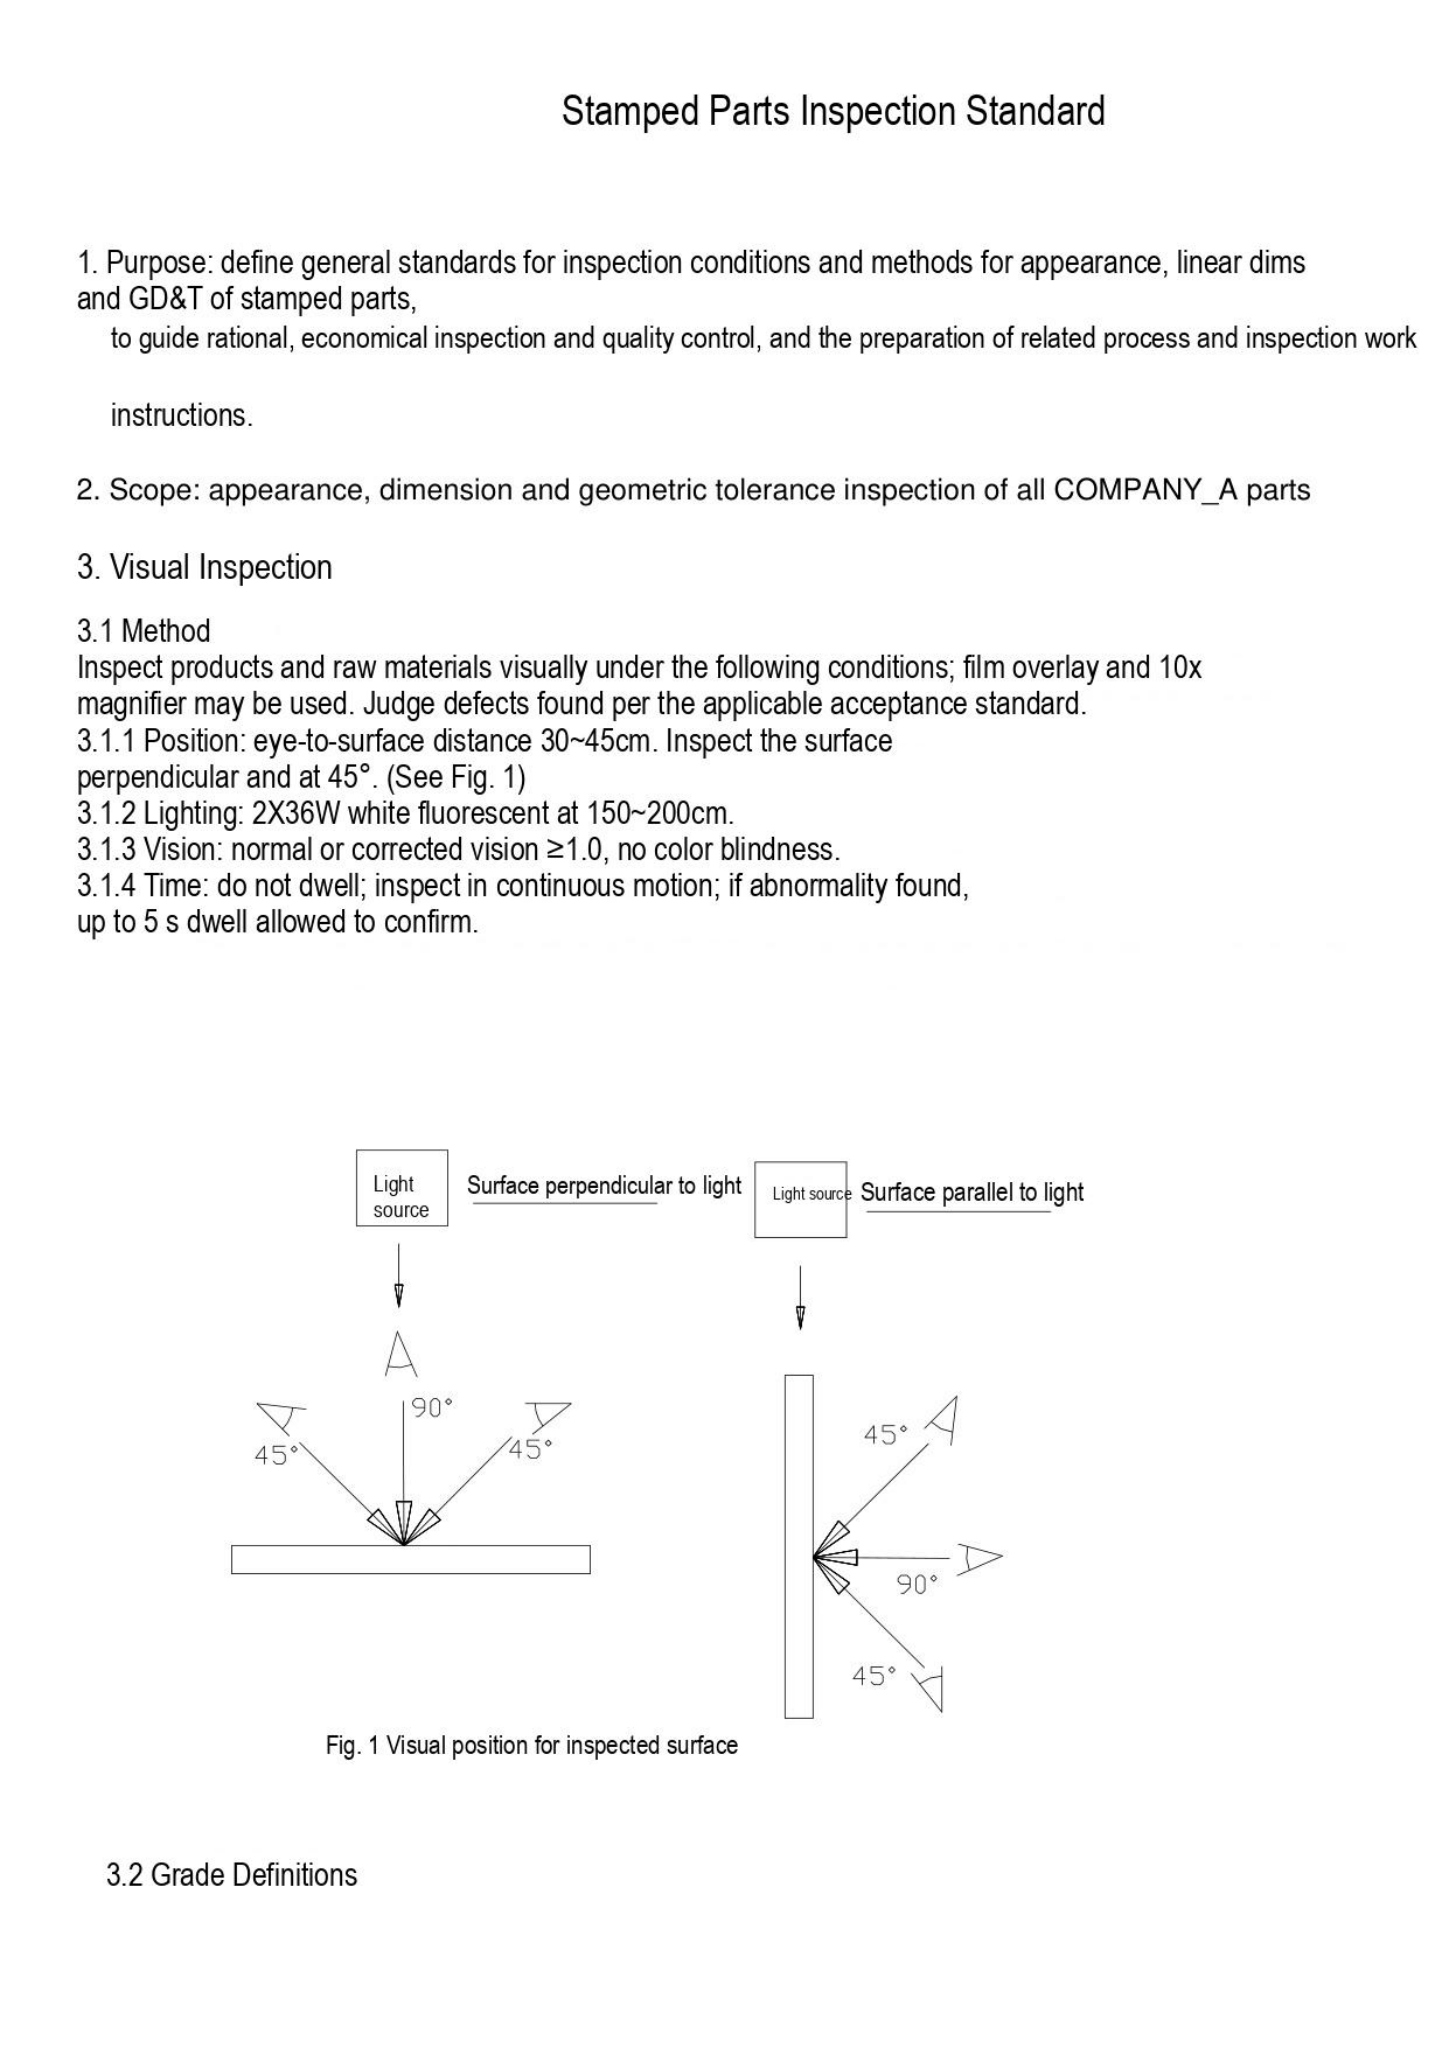Stamped Parts Inspection Standard

1. Purpose: define general standards for inspection conditions and methods for appearance, linear dims and GD&T of stamped parts,
to guide rational, economical inspection and quality control, and the preparation of related process and inspection work instructions.

2. Scope: appearance, dimension and geometric tolerance inspection of all COMPANY_A parts

3. Visual Inspection

3.1 Method
Inspect products and raw materials visually under the following conditions; film overlay and 10x magnifier may be used. Judge defects found per the applicable acceptance standard.
3.1.1 Position: eye-to-surface distance 30~45cm. Inspect the surface perpendicular and at 45°. (See Fig. 1)
3.1.2 Lighting: 2X36W white fluorescent at 150~200cm.
3.1.3 Vision: normal or corrected vision ≥1.0, no color blindness.
3.1.4 Time: do not dwell; inspect in continuous motion; if abnormality found, up to 5 s dwell allowed to confirm.

Light source
Surface perpendicular to light
90°
45°
45°

Light source
Surface parallel to light
45°
90°
45°

Fig. 1 Visual position for inspected surface

3.2 Grade Definitions
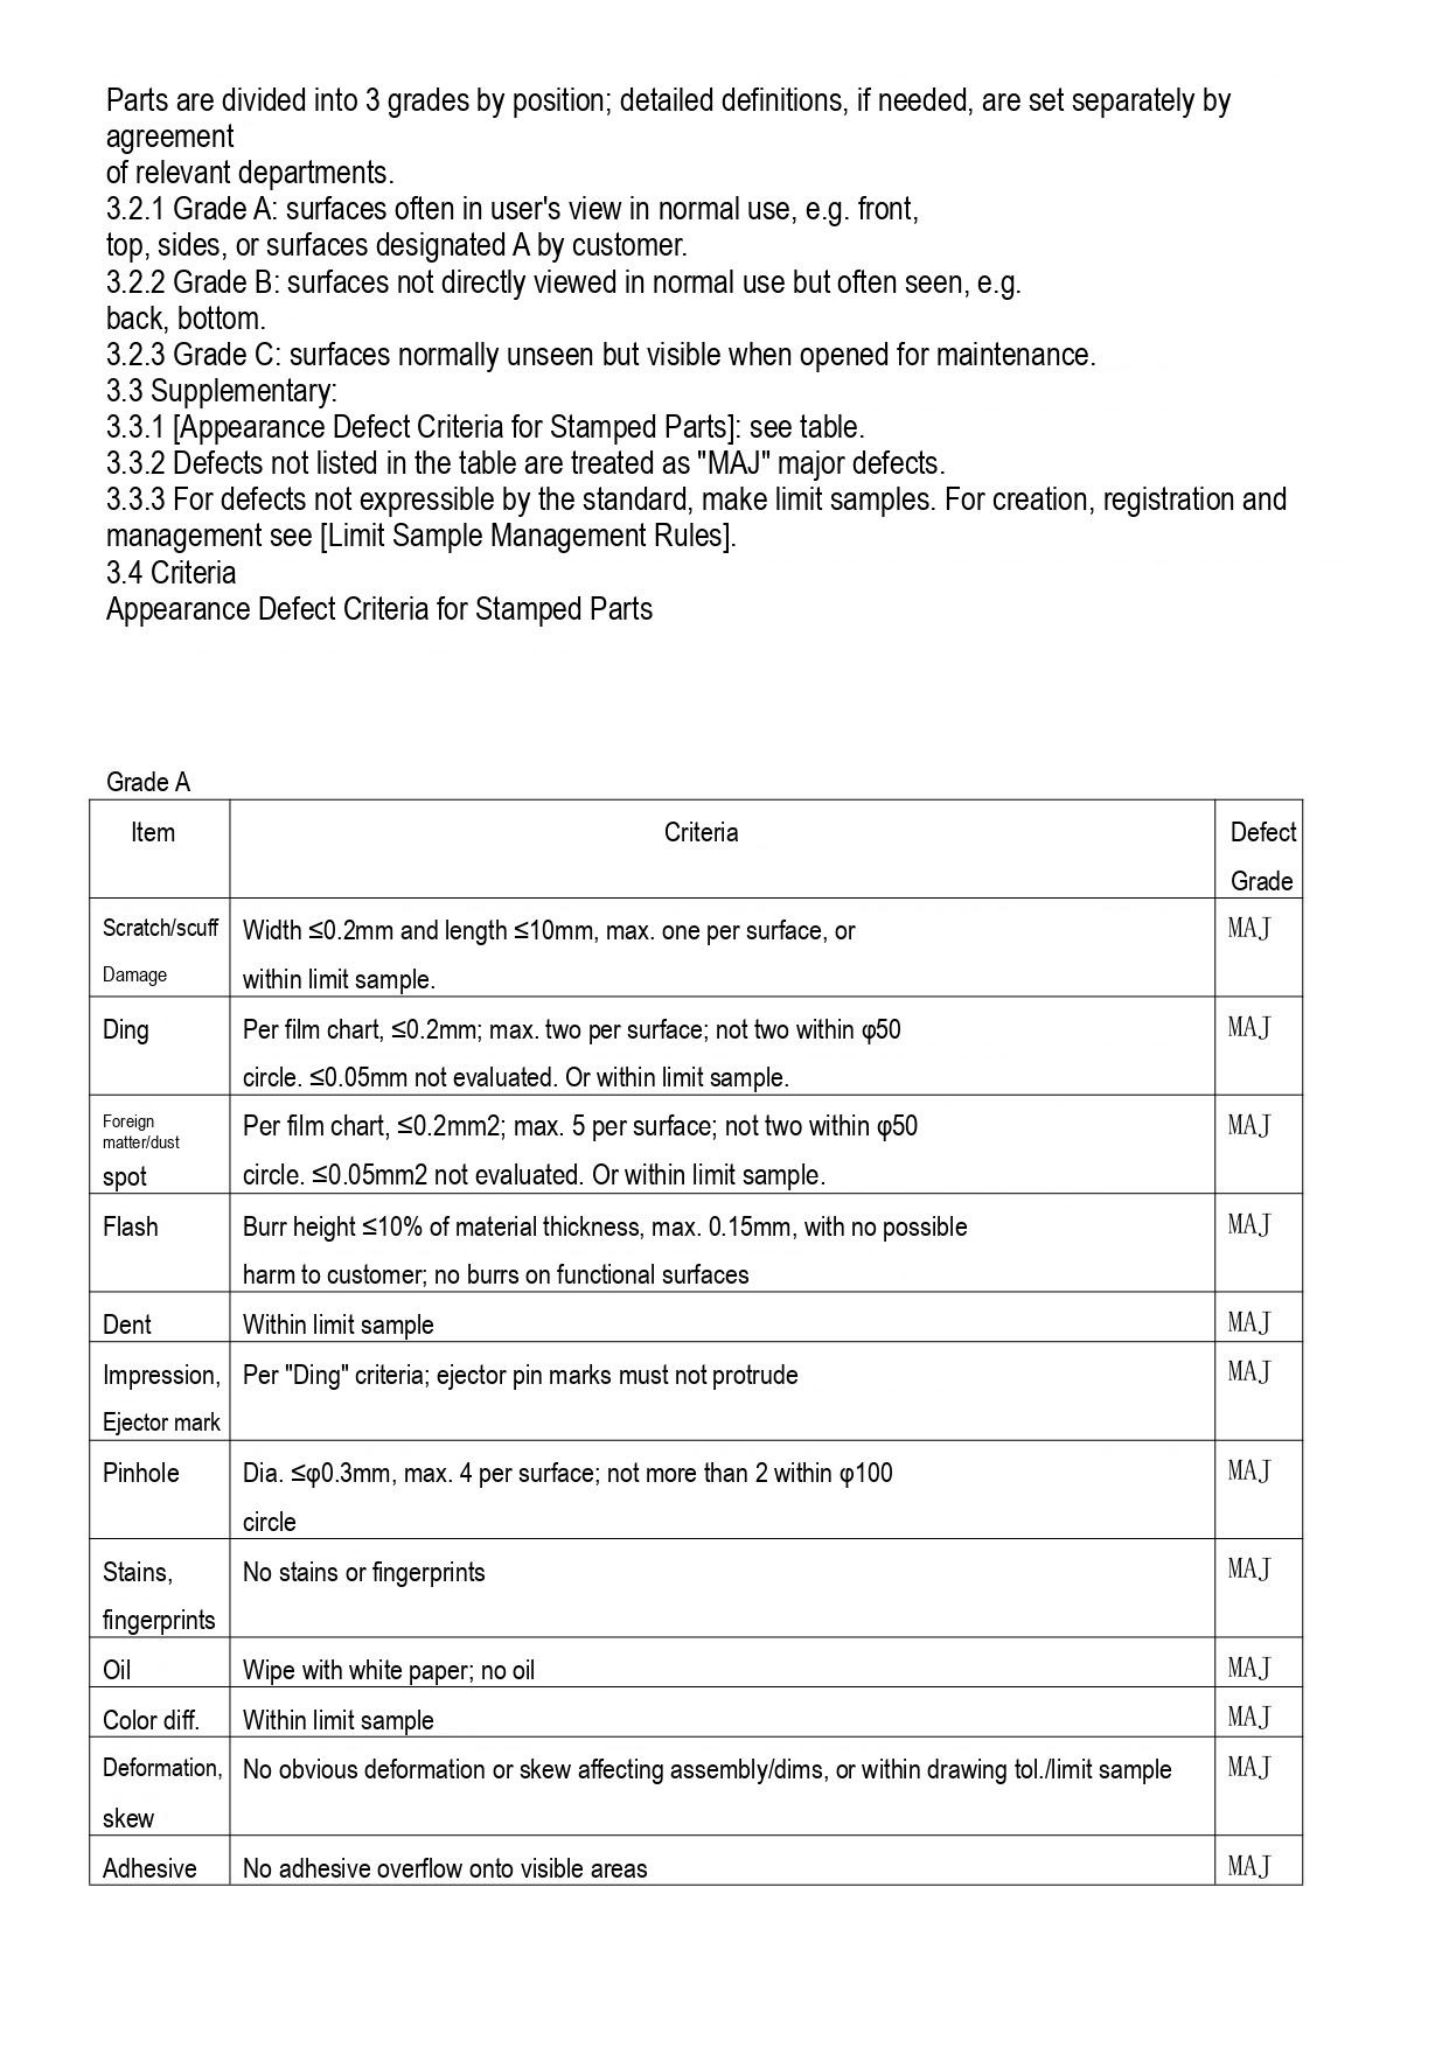Parts are divided into 3 grades by position; detailed definitions, if needed, are set separately by agreement
of relevant departments.
3.2.1 Grade A: surfaces often in user's view in normal use, e.g. front,
top, sides, or surfaces designated A by customer.
3.2.2 Grade B: surfaces not directly viewed in normal use but often seen, e.g.
back, bottom.
3.2.3 Grade C: surfaces normally unseen but visible when opened for maintenance.
3.3 Supplementary:
3.3.1 [Appearance Defect Criteria for Stamped Parts]: see table.
3.3.2 Defects not listed in the table are treated as "MAJ" major defects.
3.3.3 For defects not expressible by the standard, make limit samples. For creation, registration and management see [Limit Sample Management Rules].
3.4 Criteria
Appearance Defect Criteria for Stamped Parts

Grade A

| Item | Criteria | Defect Grade |
|---|---|---|
| Scratch/scuff Damage | Width ≤0.2mm and length ≤10mm, max. one per surface, or within limit sample. | MAJ |
| Ding | Per film chart, ≤0.2mm; max. two per surface; not two within φ50 circle. ≤0.05mm not evaluated. Or within limit sample. | MAJ |
| Foreign matter/dust spot | Per film chart, ≤0.2mm2; max. 5 per surface; not two within φ50 circle. ≤0.05mm2 not evaluated. Or within limit sample. | MAJ |
| Flash | Burr height ≤10% of material thickness, max. 0.15mm, with no possible harm to customer; no burrs on functional surfaces | MAJ |
| Dent | Within limit sample | MAJ |
| Impression, Ejector mark | Per "Ding" criteria; ejector pin marks must not protrude | MAJ |
| Pinhole | Dia. ≤φ0.3mm, max. 4 per surface; not more than 2 within φ100 circle | MAJ |
| Stains, fingerprints | No stains or fingerprints | MAJ |
| Oil | Wipe with white paper; no oil | MAJ |
| Color diff. | Within limit sample | MAJ |
| Deformation, skew | No obvious deformation or skew affecting assembly/dims, or within drawing tol./limit sample | MAJ |
| Adhesive | No adhesive overflow onto visible areas | MAJ |
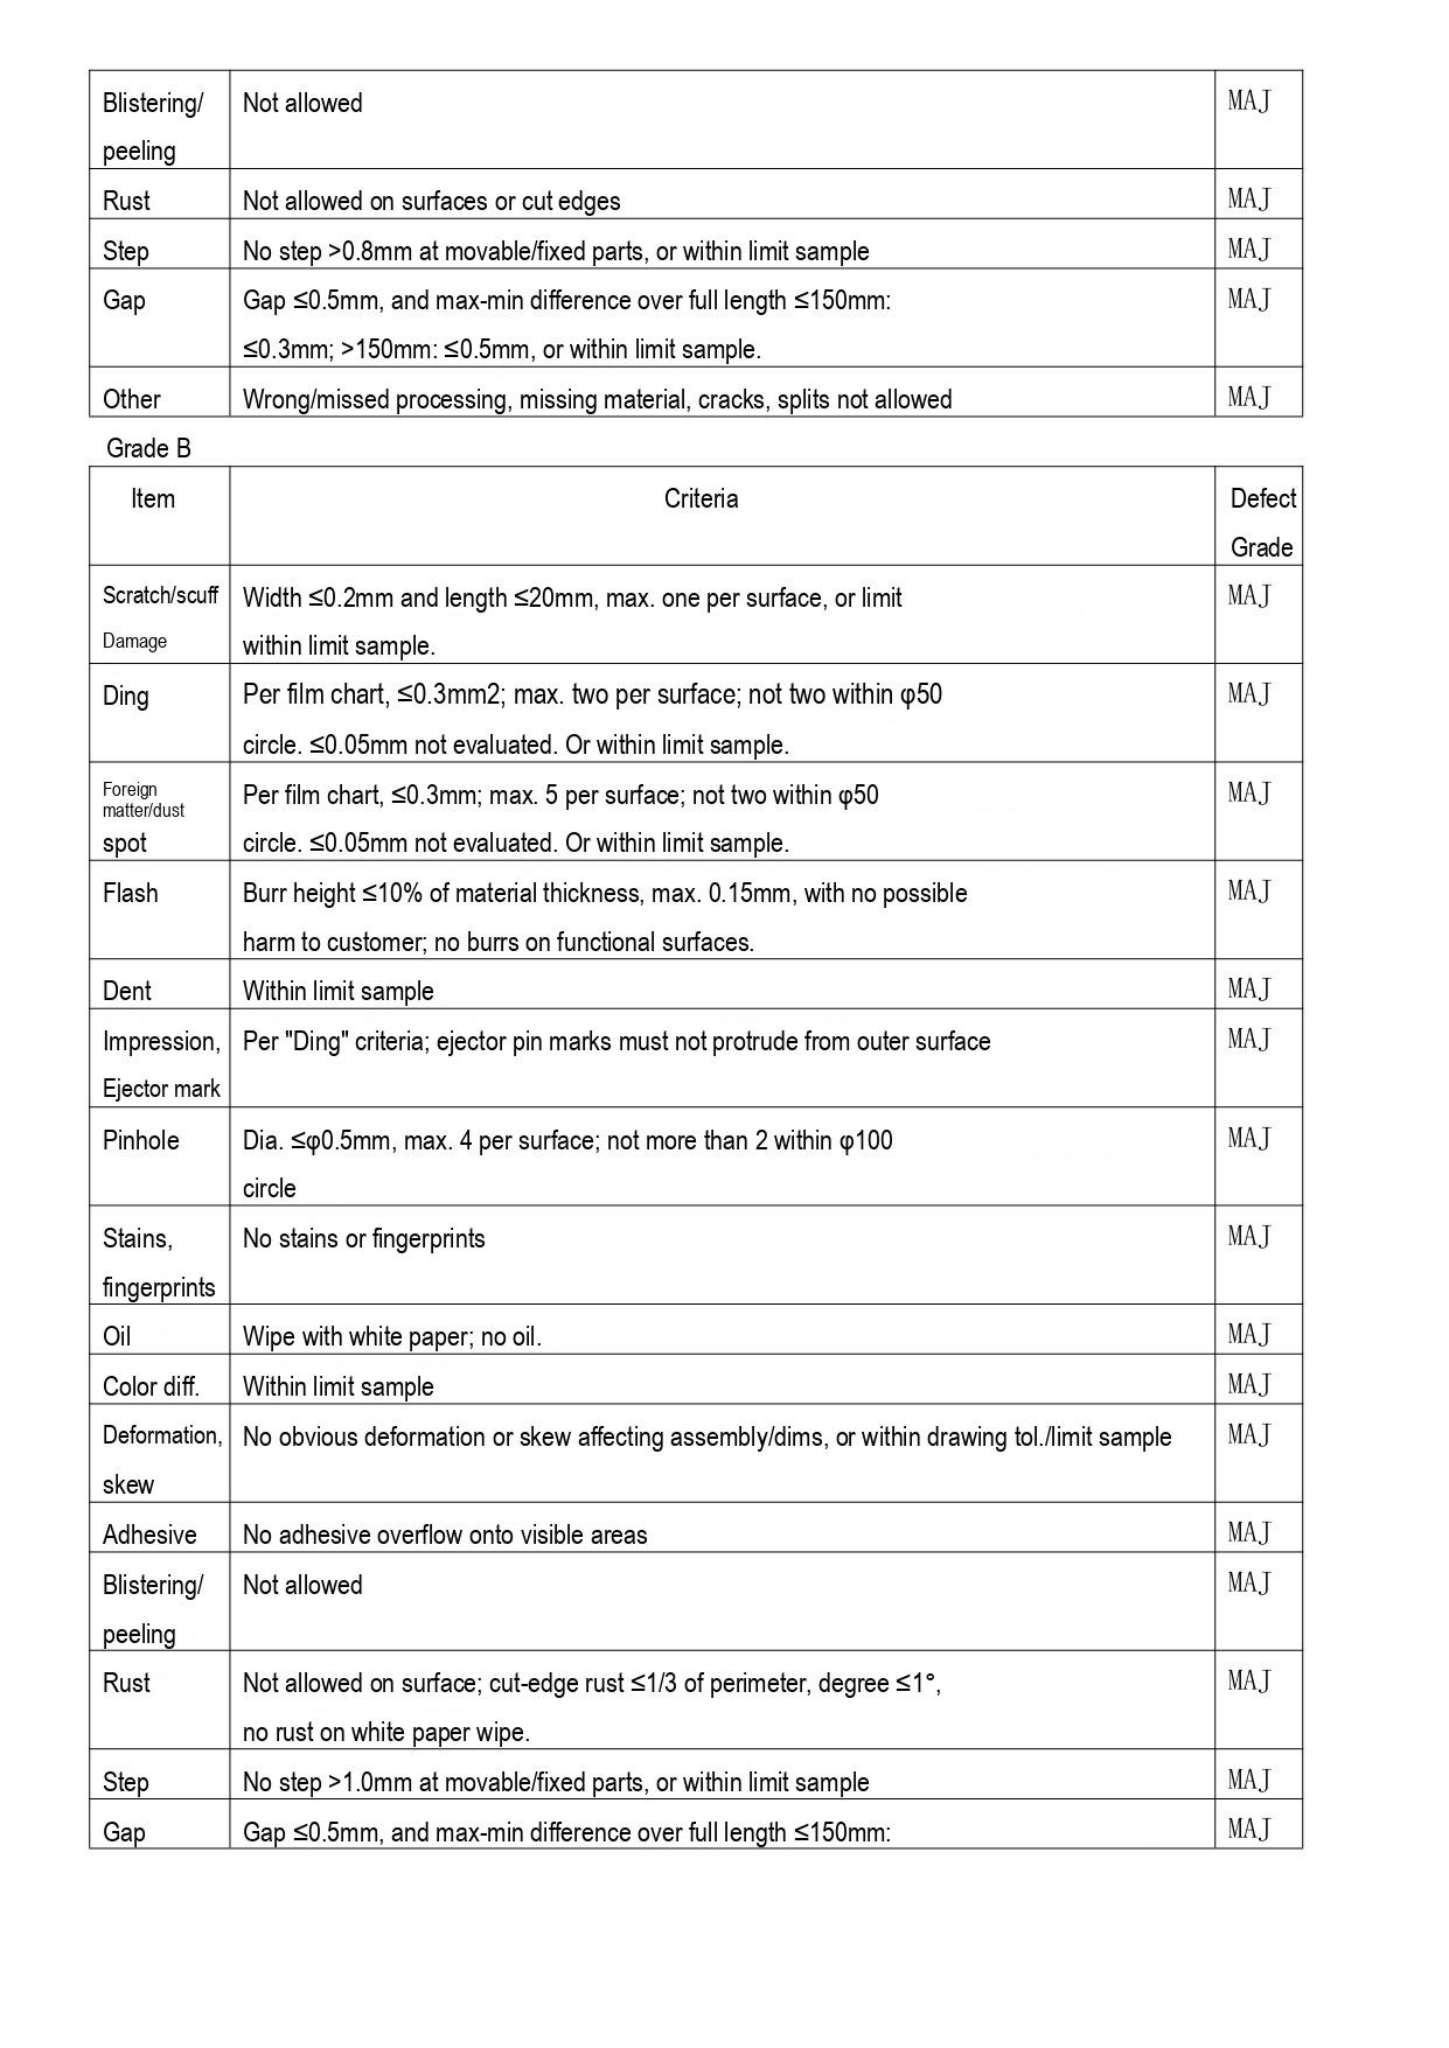| | | |
|---|---|---|
| Blistering/ peeling | Not allowed | MAJ |
| Rust | Not allowed on surfaces or cut edges | MAJ |
| Step | No step >0.8mm at movable/fixed parts, or within limit sample | MAJ |
| Gap | Gap ≤0.5mm, and max-min difference over full length ≤150mm: ≤0.3mm; >150mm: ≤0.5mm, or within limit sample. | MAJ |
| Other | Wrong/missed processing, missing material, cracks, splits not allowed | MAJ |

Grade B

| Item | Criteria | Defect Grade |
|---|---|---|
| Scratch/scuff Damage | Width ≤0.2mm and length ≤20mm, max. one per surface, or limit within limit sample. | MAJ |
| Ding | Per film chart, ≤0.3mm2; max. two per surface; not two within φ50 circle. ≤0.05mm not evaluated. Or within limit sample. | MAJ |
| Foreign matter/dust spot | Per film chart, ≤0.3mm; max. 5 per surface; not two within φ50 circle. ≤0.05mm not evaluated. Or within limit sample. | MAJ |
| Flash | Burr height ≤10% of material thickness, max. 0.15mm, with no possible harm to customer; no burrs on functional surfaces. | MAJ |
| Dent | Within limit sample | MAJ |
| Impression, Ejector mark | Per "Ding" criteria; ejector pin marks must not protrude from outer surface | MAJ |
| Pinhole | Dia. ≤φ0.5mm, max. 4 per surface; not more than 2 within φ100 circle | MAJ |
| Stains, fingerprints | No stains or fingerprints | MAJ |
| Oil | Wipe with white paper; no oil. | MAJ |
| Color diff. | Within limit sample | MAJ |
| Deformation, skew | No obvious deformation or skew affecting assembly/dims, or within drawing tol./limit sample | MAJ |
| Adhesive | No adhesive overflow onto visible areas | MAJ |
| Blistering/ peeling | Not allowed | MAJ |
| Rust | Not allowed on surface; cut-edge rust ≤1/3 of perimeter, degree ≤1°, no rust on white paper wipe. | MAJ |
| Step | No step >1.0mm at movable/fixed parts, or within limit sample | MAJ |
| Gap | Gap ≤0.5mm, and max-min difference over full length ≤150mm: | MAJ |
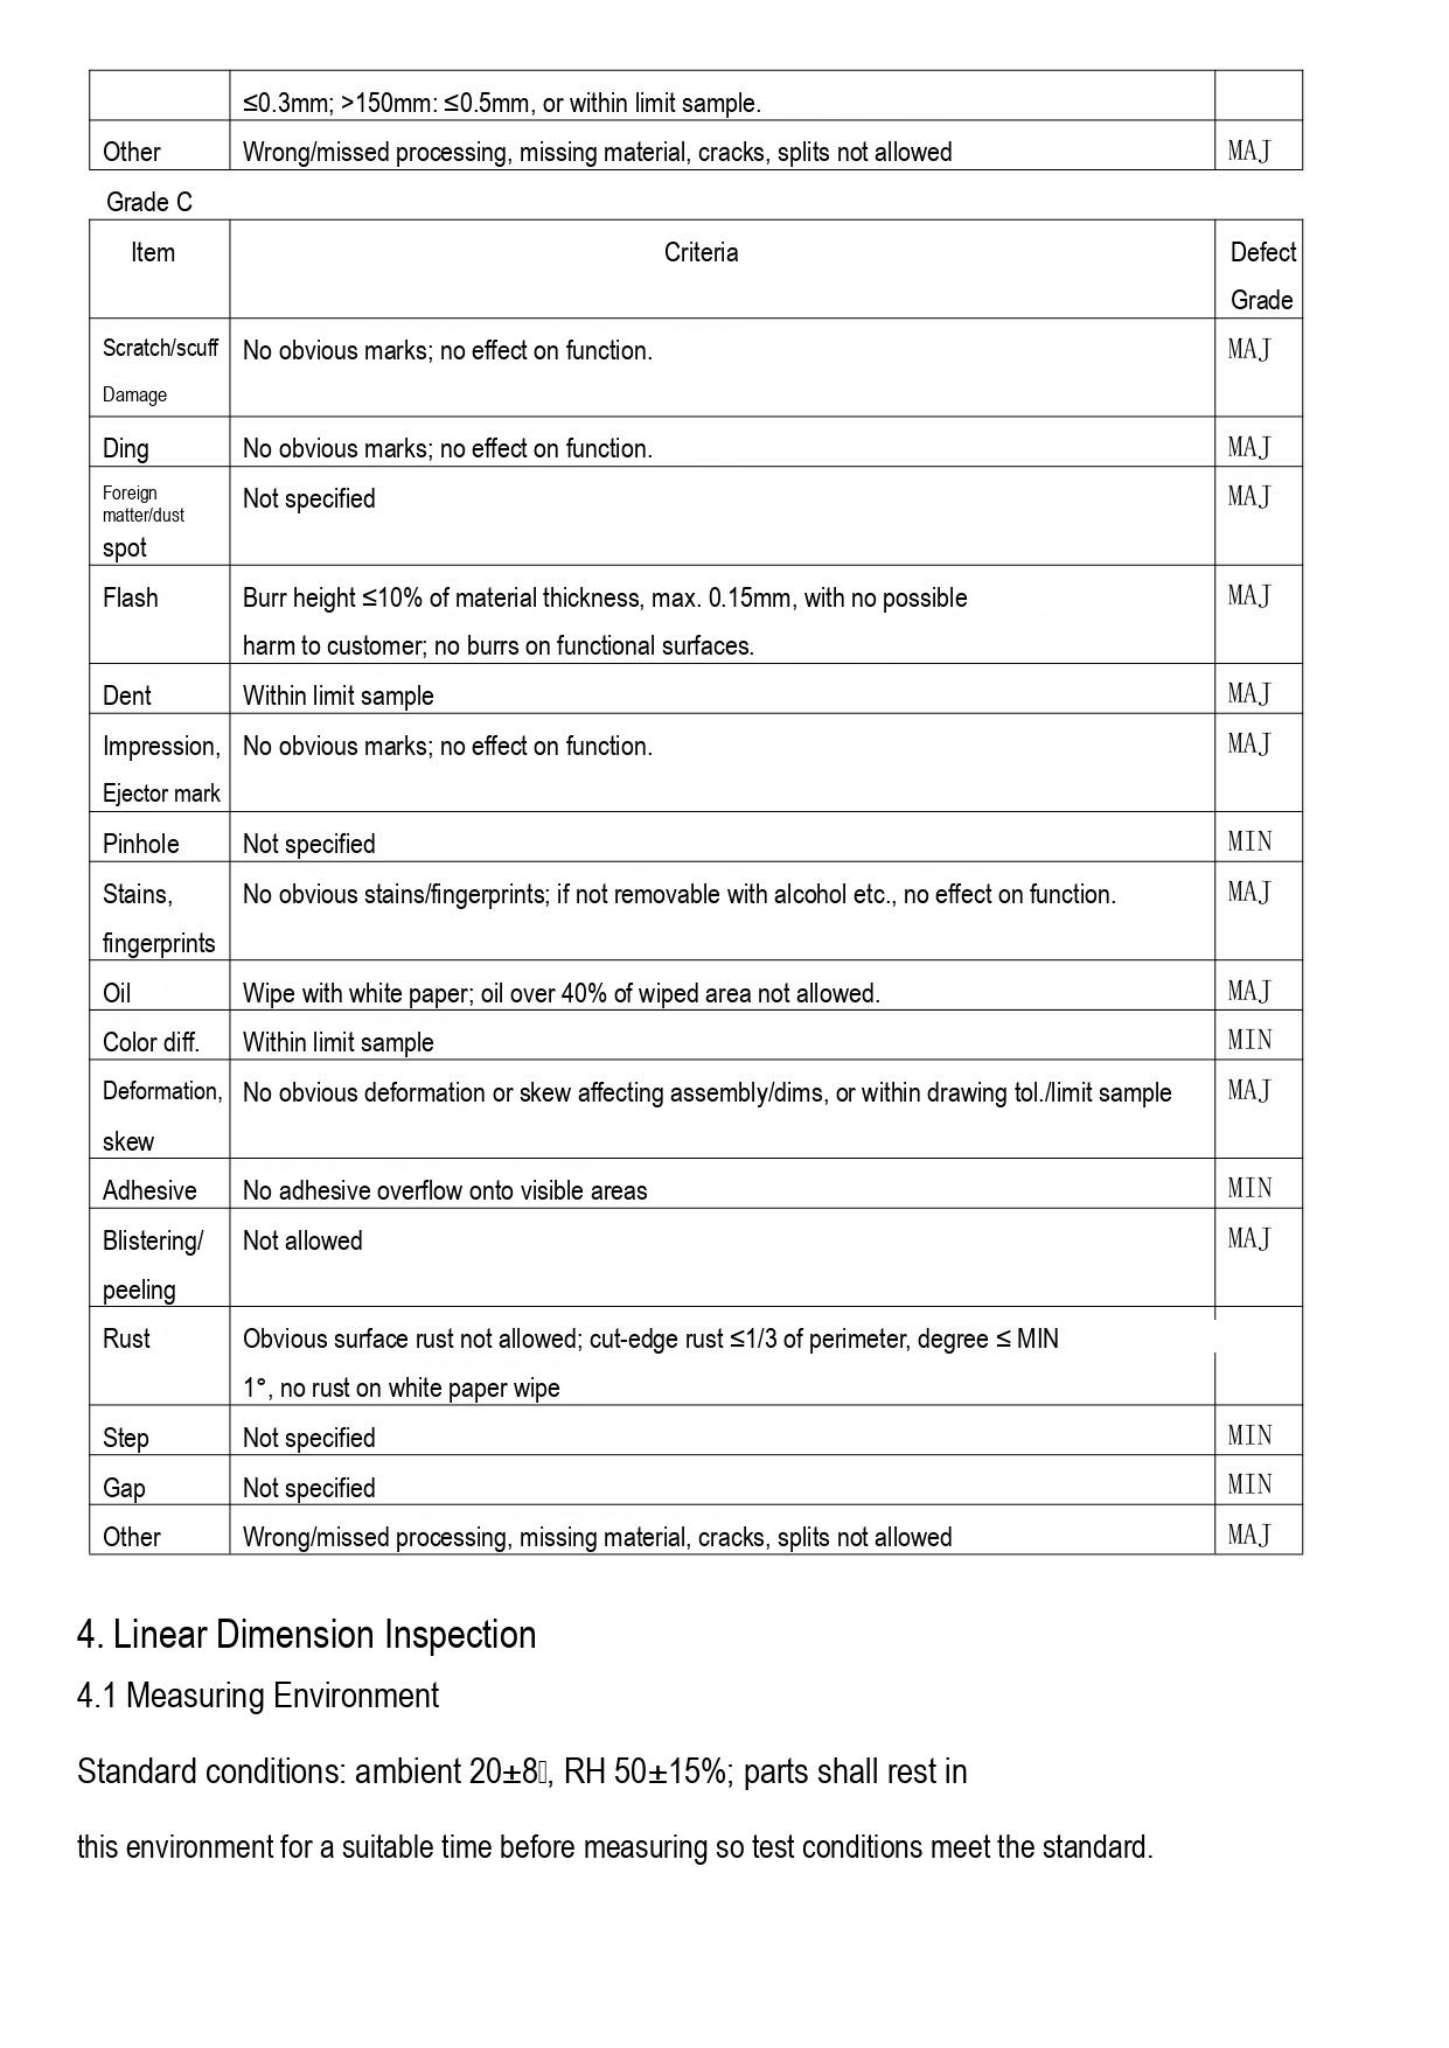| | ≤0.3mm; >150mm: ≤0.5mm, or within limit sample. | |
|---|---|---|
| Other | Wrong/missed processing, missing material, cracks, splits not allowed | MAJ |

Grade C

| Item | Criteria | Defect Grade |
|---|---|---|
| Scratch/scuff Damage | No obvious marks; no effect on function. | MAJ |
| Ding | No obvious marks; no effect on function. | MAJ |
| Foreign matter/dust spot | Not specified | MAJ |
| Flash | Burr height ≤10% of material thickness, max. 0.15mm, with no possible harm to customer; no burrs on functional surfaces. | MAJ |
| Dent | Within limit sample | MAJ |
| Impression, Ejector mark | No obvious marks; no effect on function. | MAJ |
| Pinhole | Not specified | MIN |
| Stains, fingerprints | No obvious stains/fingerprints; if not removable with alcohol etc., no effect on function. | MAJ |
| Oil | Wipe with white paper; oil over 40% of wiped area not allowed. | MAJ |
| Color diff. | Within limit sample | MIN |
| Deformation, skew | No obvious deformation or skew affecting assembly/dims, or within drawing tol./limit sample | MAJ |
| Adhesive | No adhesive overflow onto visible areas | MIN |
| Blistering/ peeling | Not allowed | MAJ |
| Rust | Obvious surface rust not allowed; cut-edge rust ≤1/3 of perimeter, degree ≤ MIN 1°, no rust on white paper wipe | |
| Step | Not specified | MIN |
| Gap | Not specified | MIN |
| Other | Wrong/missed processing, missing material, cracks, splits not allowed | MAJ |

4. Linear Dimension Inspection

4.1 Measuring Environment

Standard conditions: ambient 20±8, RH 50±15%; parts shall rest in

this environment for a suitable time before measuring so test conditions meet the standard.
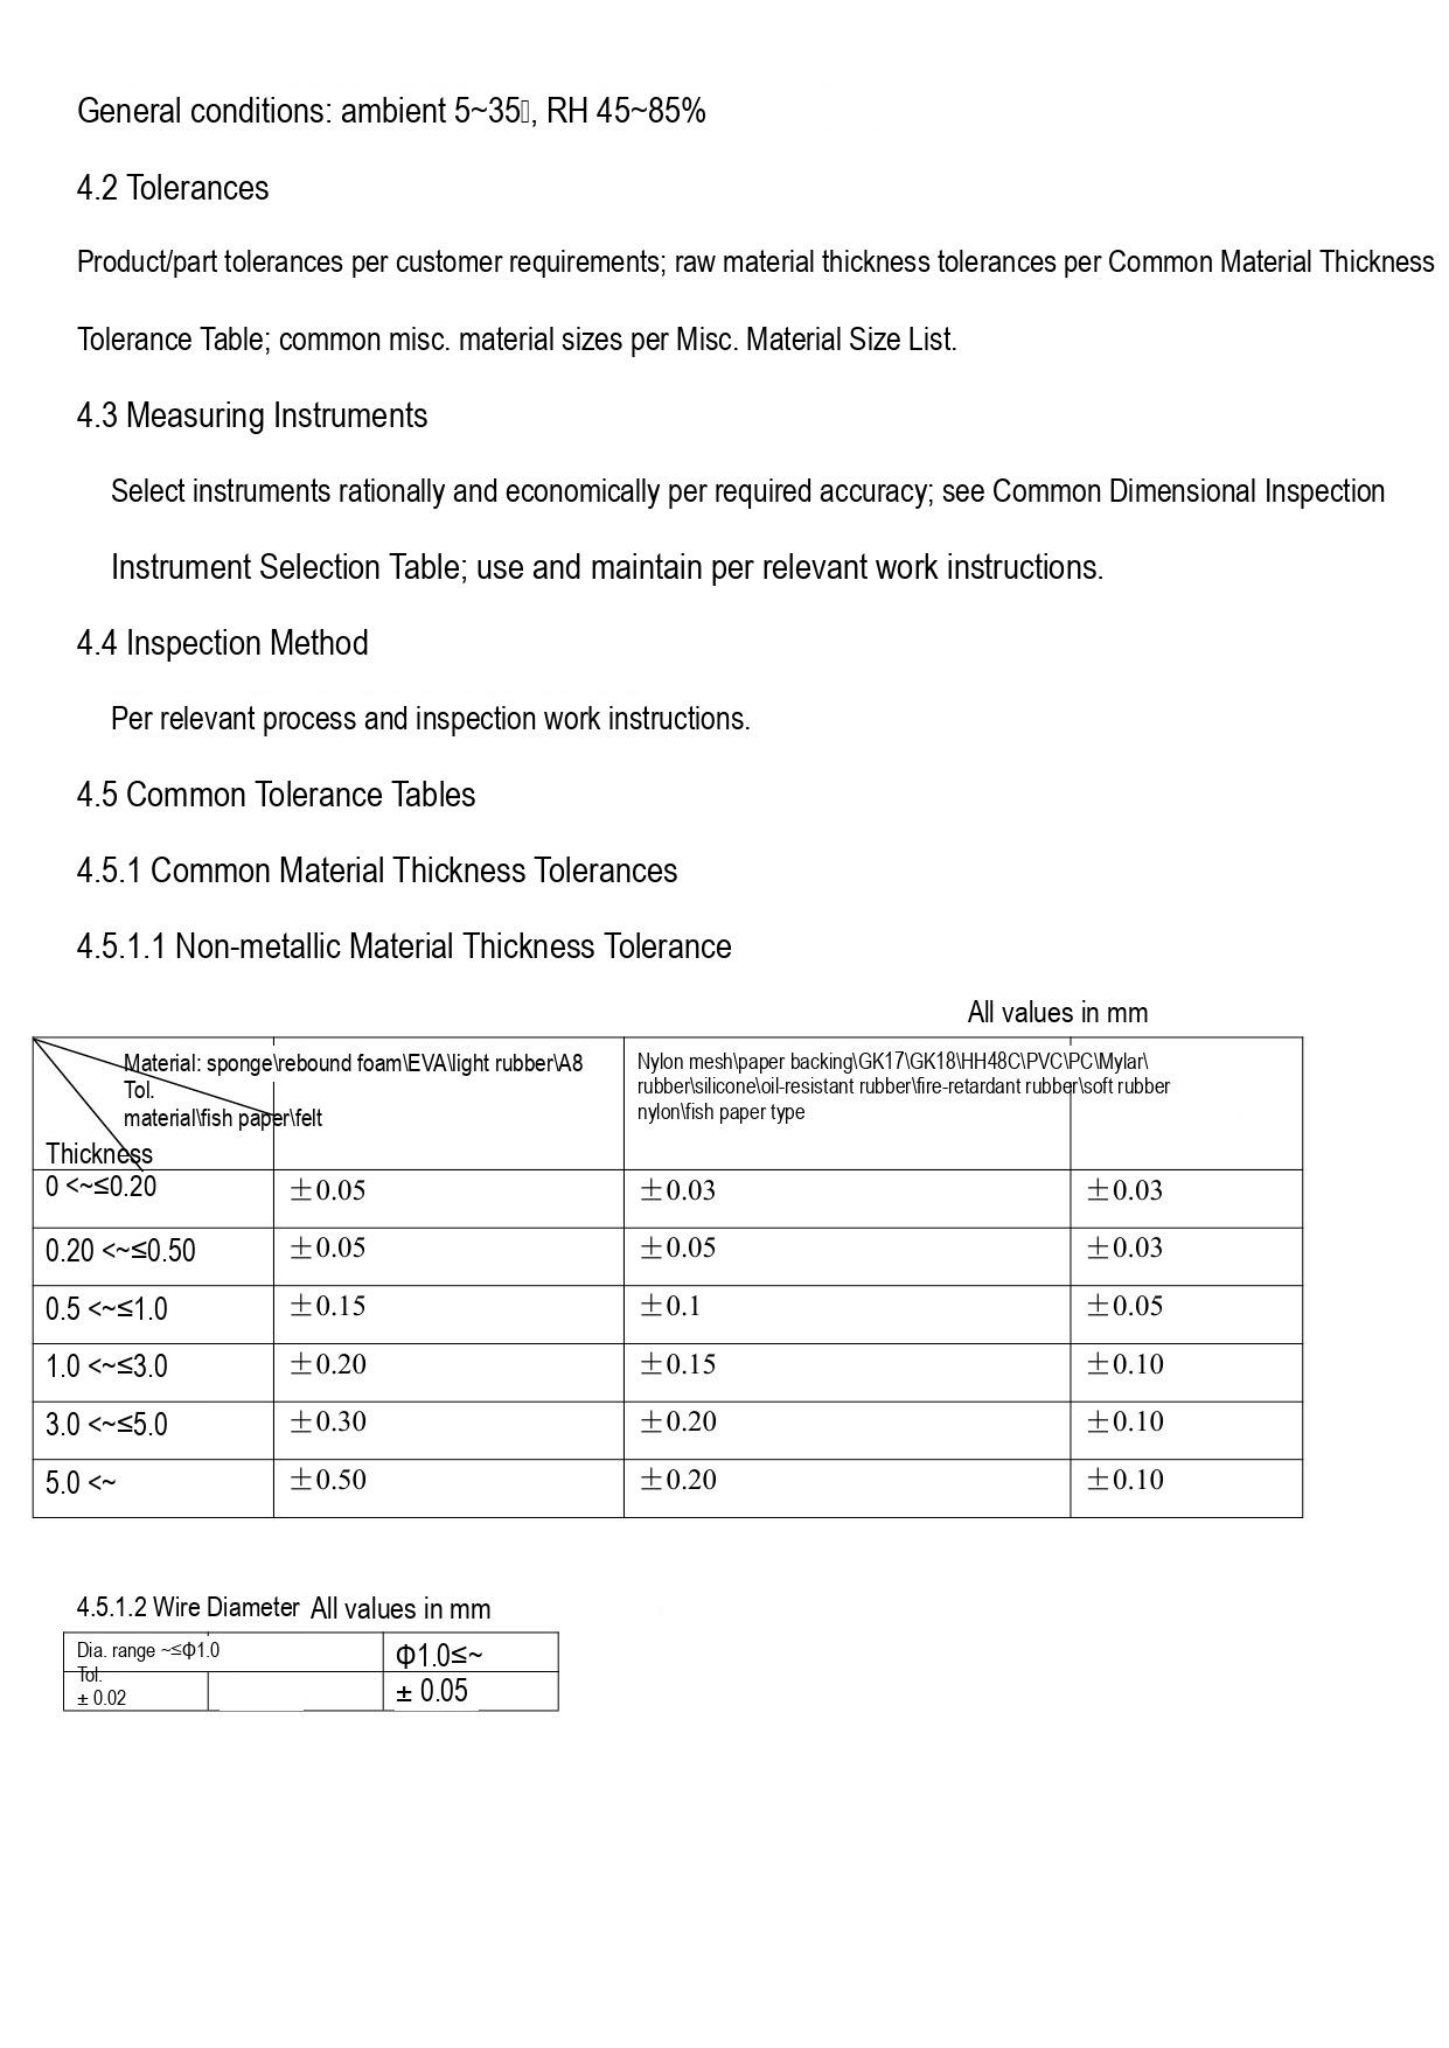General conditions: ambient 5~35, RH 45~85%

4.2 Tolerances

Product/part tolerances per customer requirements; raw material thickness tolerances per Common Material Thickness Tolerance Table; common misc. material sizes per Misc. Material Size List.

4.3 Measuring Instruments

Select instruments rationally and economically per required accuracy; see Common Dimensional Inspection Instrument Selection Table; use and maintain per relevant work instructions.

4.4 Inspection Method

Per relevant process and inspection work instructions.

4.5 Common Tolerance Tables

4.5.1 Common Material Thickness Tolerances

4.5.1.1 Non-metallic Material Thickness Tolerance

All values in mm

| Material: sponge\rebound foam\EVA\light rubber\A8 material\fish paper\felt<br>Tol.<br>Thickness | | Nylon mesh\paper backing\GK17\GK18\HH48C\PVC\PC\Mylar\ rubber\silicone\oil-resistant rubber\fire-retardant rubber\soft rubber nylon\fish paper type | |
|---|---|---|---|
| 0 <~≤0.20 | ±0.05 | ±0.03 | ±0.03 |
| 0.20 <~≤0.50 | ±0.05 | ±0.05 | ±0.03 |
| 0.5 <~≤1.0 | ±0.15 | ±0.1 | ±0.05 |
| 1.0 <~≤3.0 | ±0.20 | ±0.15 | ±0.10 |
| 3.0 <~≤5.0 | ±0.30 | ±0.20 | ±0.10 |
| 5.0 <~ | ±0.50 | ±0.20 | ±0.10 |

4.5.1.2 Wire Diameter All values in mm

| Dia. range ~≤Φ1.0<br>Tol. | | Φ1.0≤~ |
|---|---|---|
| ± 0.02 | | ± 0.05 |
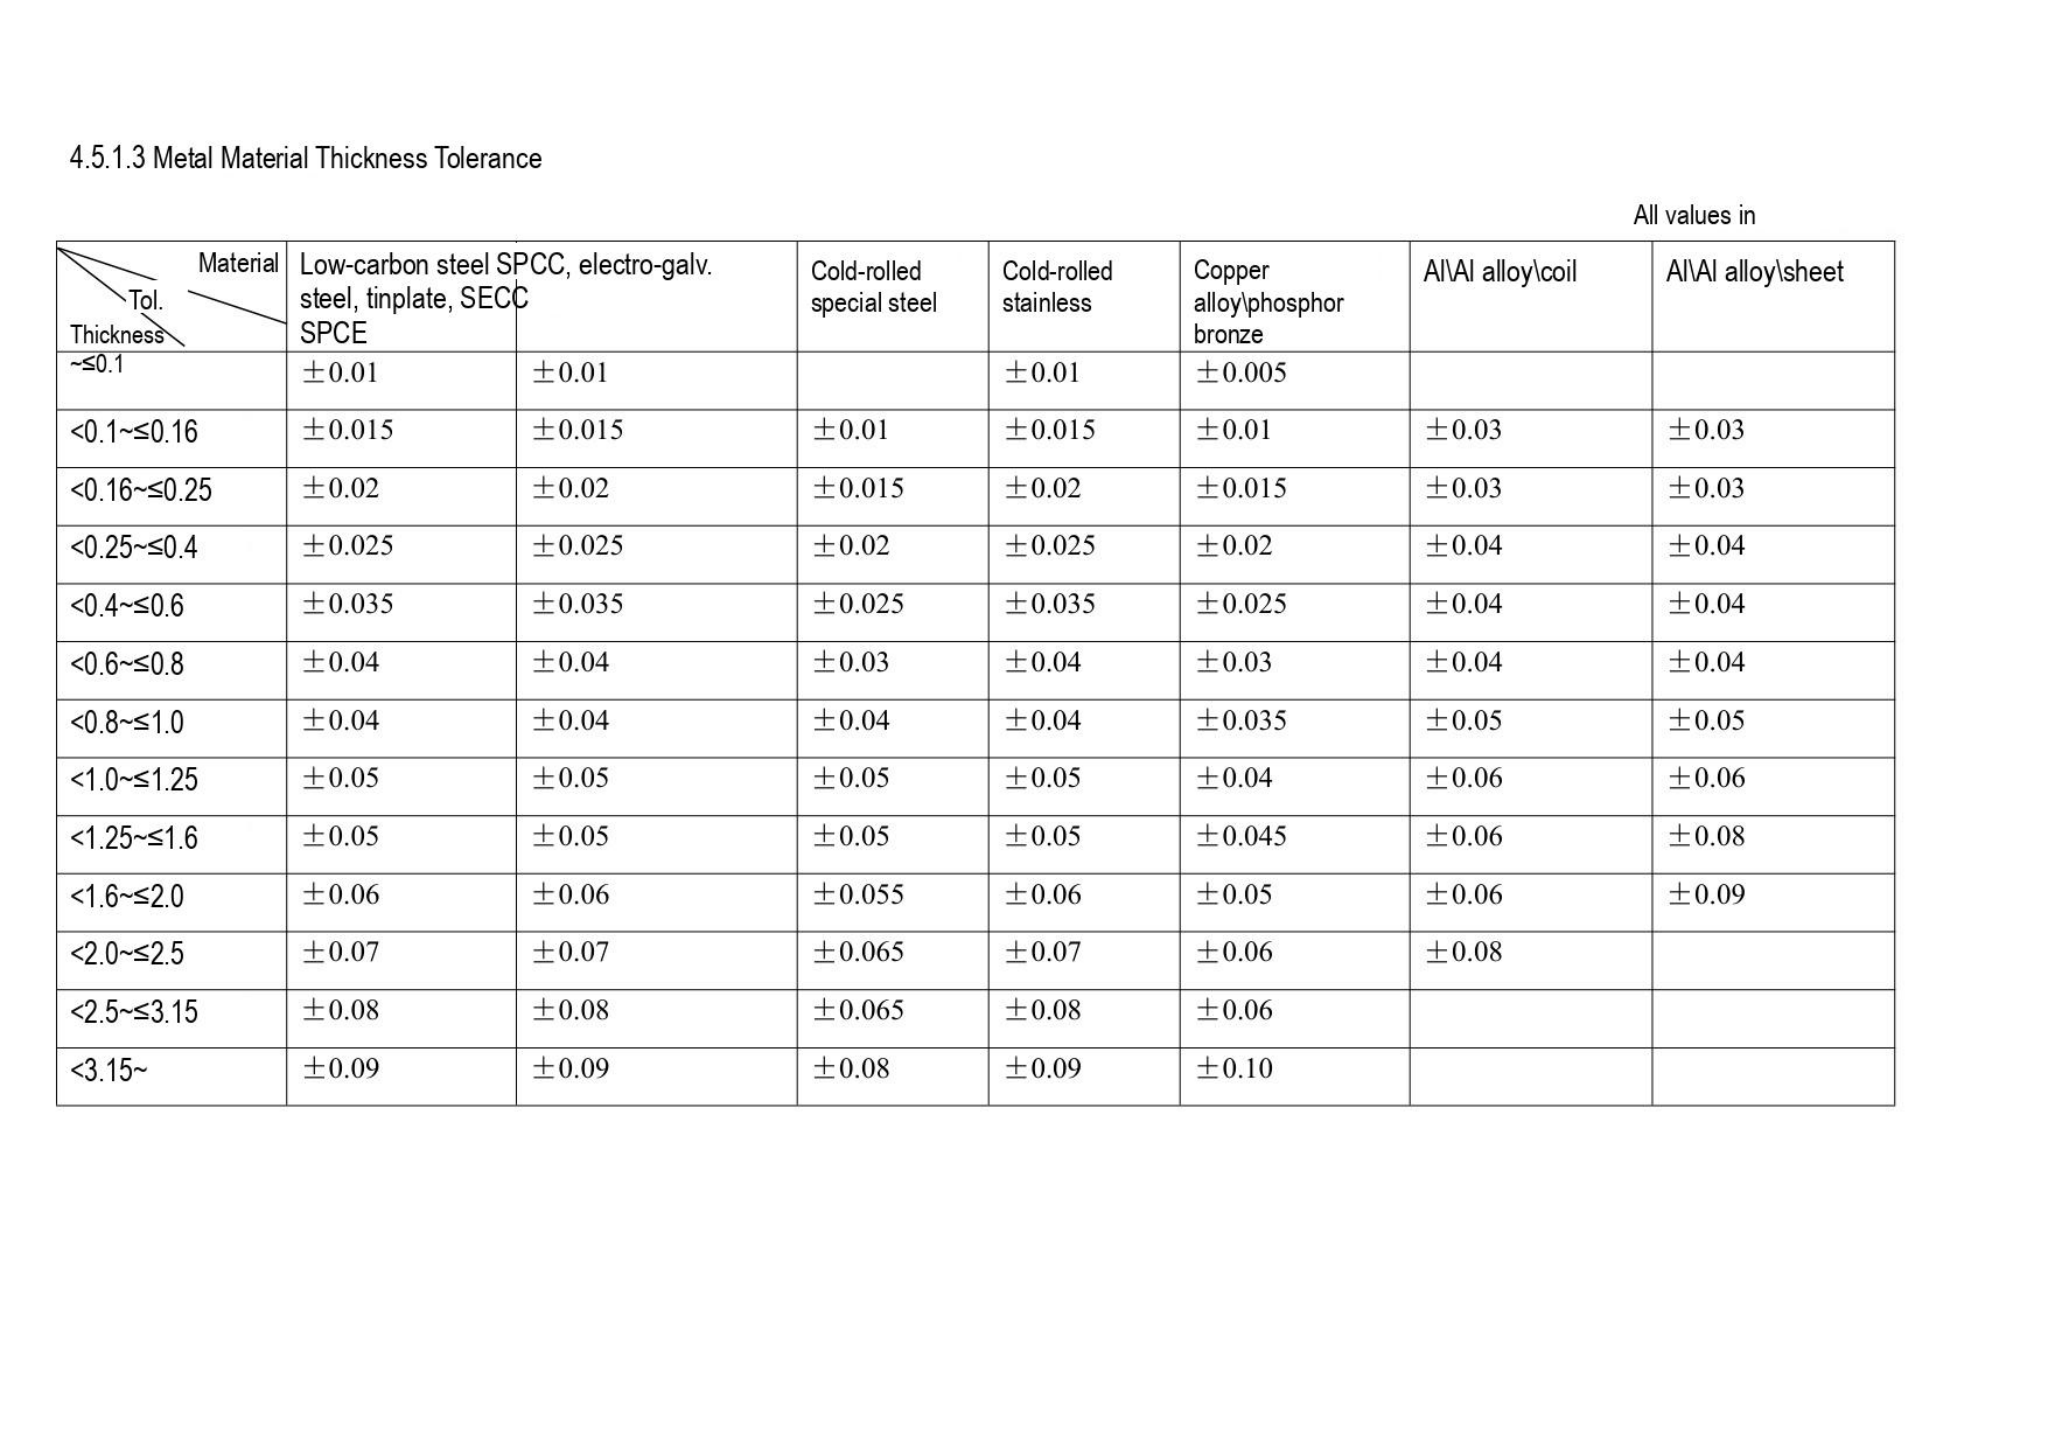4.5.1.3 Metal Material Thickness Tolerance

All values in

| Material Tol. Thickness | Low-carbon steel SPCC, electro-galv. steel, tinplate, SECC SPCE | | Cold-rolled special steel | Cold-rolled stainless | Copper alloy\phosphor bronze | Al\Al alloy\coil | Al\Al alloy\sheet |
|---|---|---|---|---|---|---|---|
| ~≤0.1 | ±0.01 | ±0.01 | | ±0.01 | ±0.005 | | |
| <0.1~≤0.16 | ±0.015 | ±0.015 | ±0.01 | ±0.015 | ±0.01 | ±0.03 | ±0.03 |
| <0.16~≤0.25 | ±0.02 | ±0.02 | ±0.015 | ±0.02 | ±0.015 | ±0.03 | ±0.03 |
| <0.25~≤0.4 | ±0.025 | ±0.025 | ±0.02 | ±0.025 | ±0.02 | ±0.04 | ±0.04 |
| <0.4~≤0.6 | ±0.035 | ±0.035 | ±0.025 | ±0.035 | ±0.025 | ±0.04 | ±0.04 |
| <0.6~≤0.8 | ±0.04 | ±0.04 | ±0.03 | ±0.04 | ±0.03 | ±0.04 | ±0.04 |
| <0.8~≤1.0 | ±0.04 | ±0.04 | ±0.04 | ±0.04 | ±0.035 | ±0.05 | ±0.05 |
| <1.0~≤1.25 | ±0.05 | ±0.05 | ±0.05 | ±0.05 | ±0.04 | ±0.06 | ±0.06 |
| <1.25~≤1.6 | ±0.05 | ±0.05 | ±0.05 | ±0.05 | ±0.045 | ±0.06 | ±0.08 |
| <1.6~≤2.0 | ±0.06 | ±0.06 | ±0.055 | ±0.06 | ±0.05 | ±0.06 | ±0.09 |
| <2.0~≤2.5 | ±0.07 | ±0.07 | ±0.065 | ±0.07 | ±0.06 | ±0.08 | |
| <2.5~≤3.15 | ±0.08 | ±0.08 | ±0.065 | ±0.08 | ±0.06 | | |
| <3.15~ | ±0.09 | ±0.09 | ±0.08 | ±0.09 | ±0.10 | | |
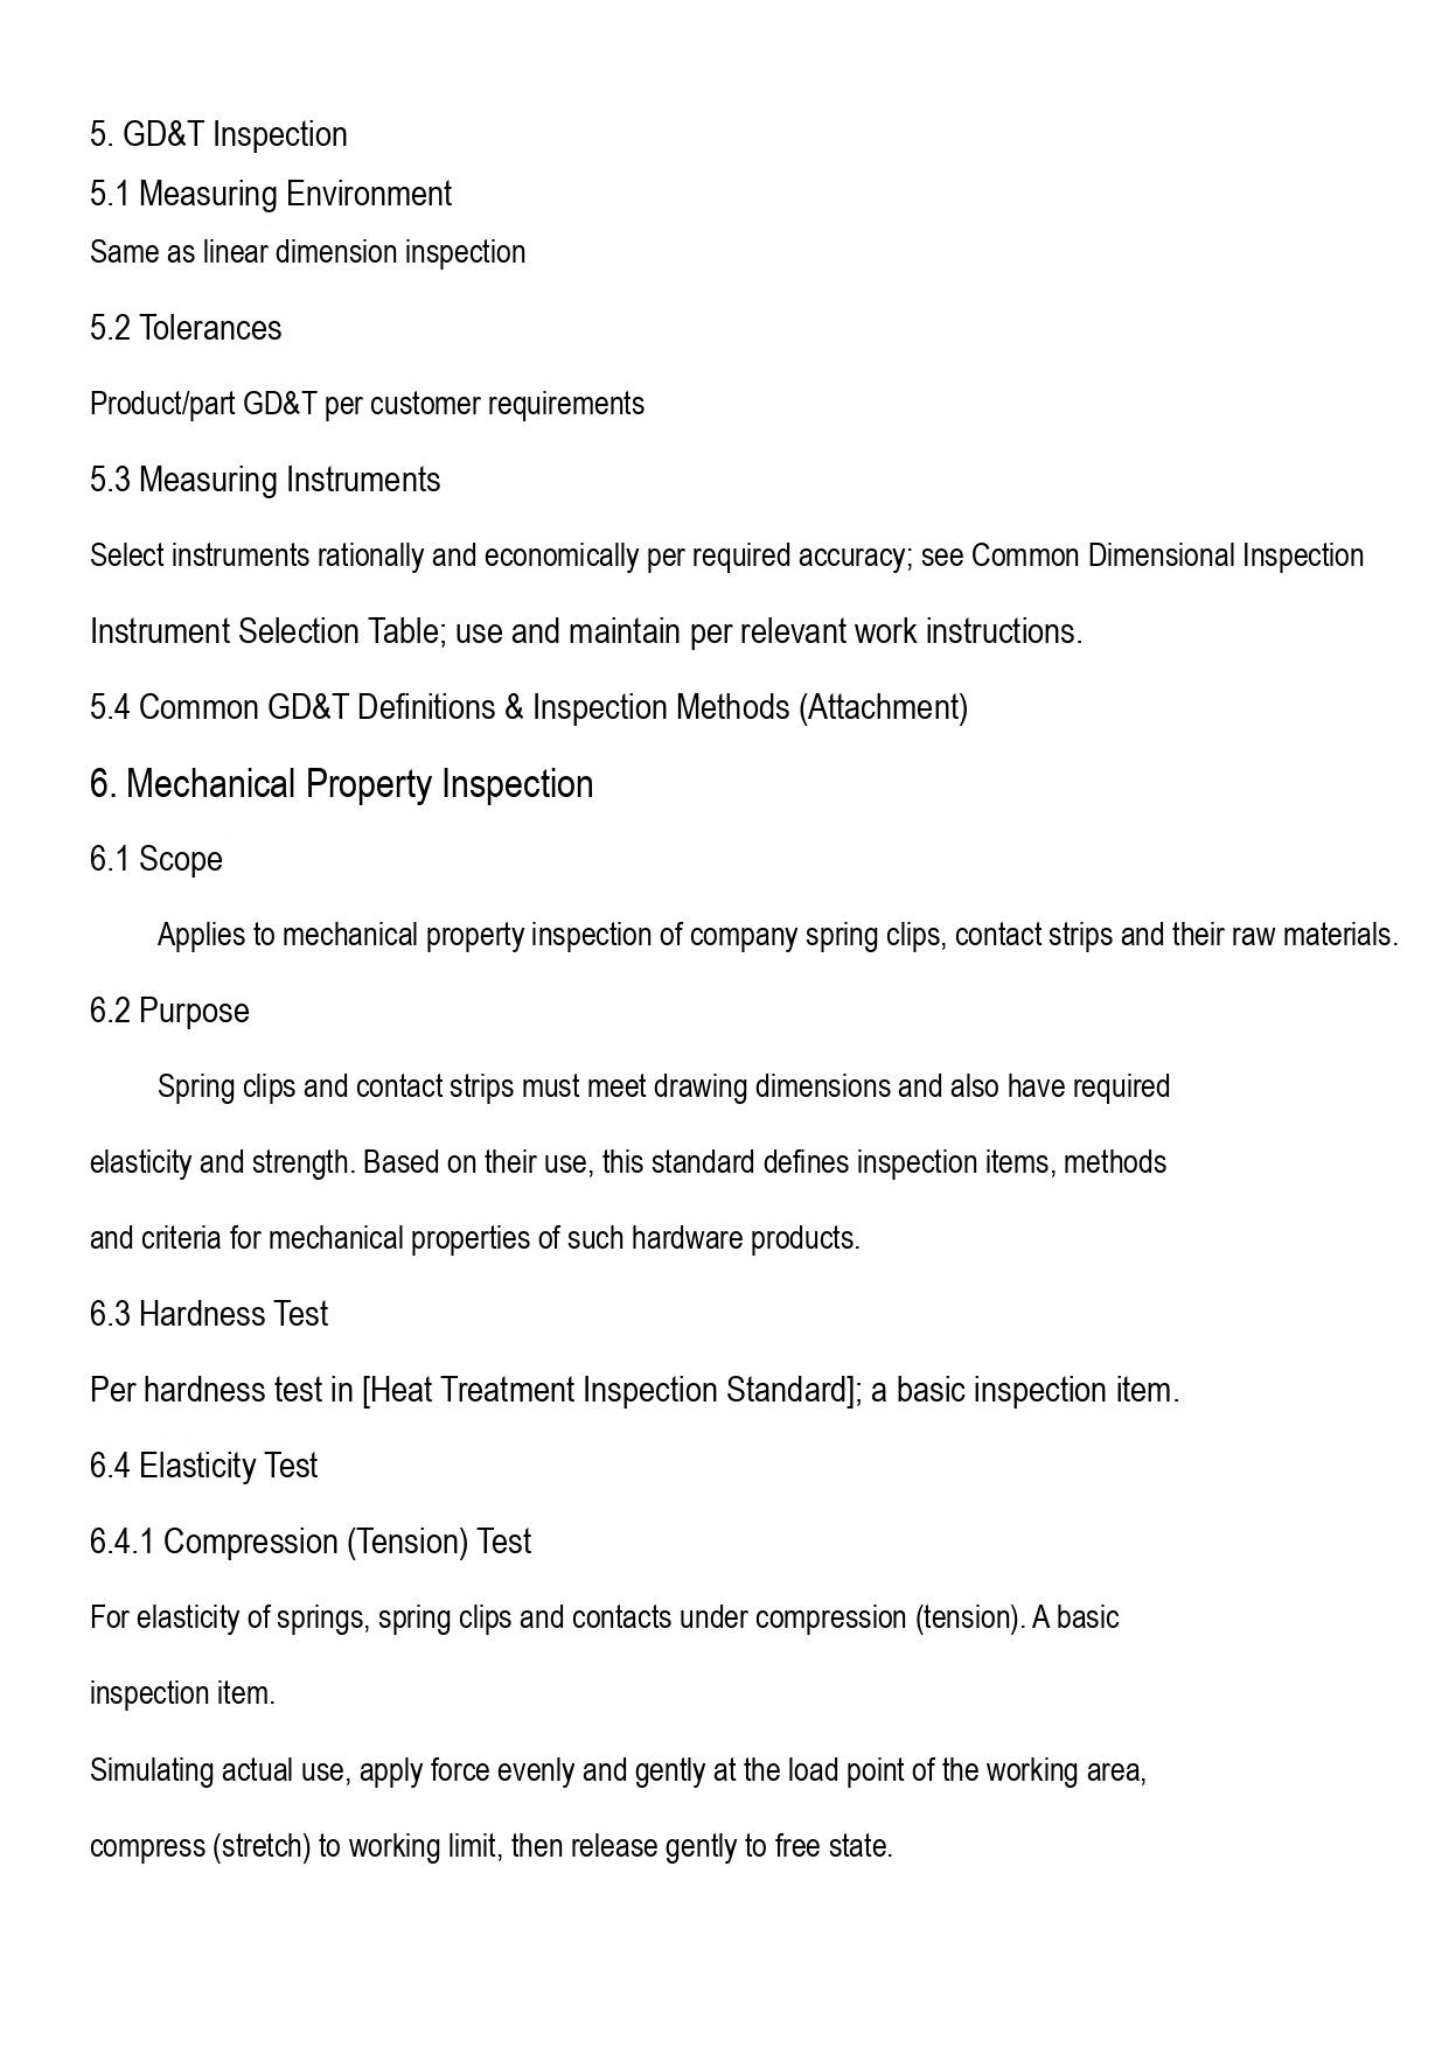5. GD&T Inspection

5.1 Measuring Environment

Same as linear dimension inspection

5.2 Tolerances

Product/part GD&T per customer requirements

5.3 Measuring Instruments

Select instruments rationally and economically per required accuracy; see Common Dimensional Inspection Instrument Selection Table; use and maintain per relevant work instructions.

5.4 Common GD&T Definitions & Inspection Methods (Attachment)

6. Mechanical Property Inspection

6.1 Scope

Applies to mechanical property inspection of company spring clips, contact strips and their raw materials.

6.2 Purpose

Spring clips and contact strips must meet drawing dimensions and also have required elasticity and strength. Based on their use, this standard defines inspection items, methods and criteria for mechanical properties of such hardware products.

6.3 Hardness Test

Per hardness test in [Heat Treatment Inspection Standard]; a basic inspection item.

6.4 Elasticity Test

6.4.1 Compression (Tension) Test

For elasticity of springs, spring clips and contacts under compression (tension). A basic inspection item.

Simulating actual use, apply force evenly and gently at the load point of the working area, compress (stretch) to working limit, then release gently to free state.